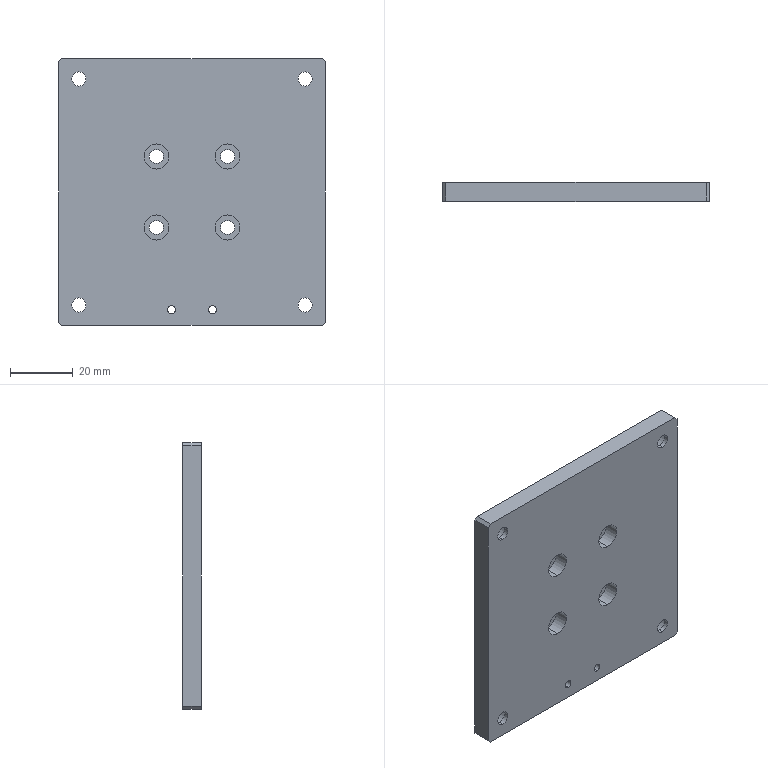Part | STEP file | 1 solid | 54 faces | box 85 x 6 x 85 mm | volume 41251 mm3 | cylinder 36 | plane 18 | commonest cylinder face diameters 4.5 x16 8 x16 2.5 x4